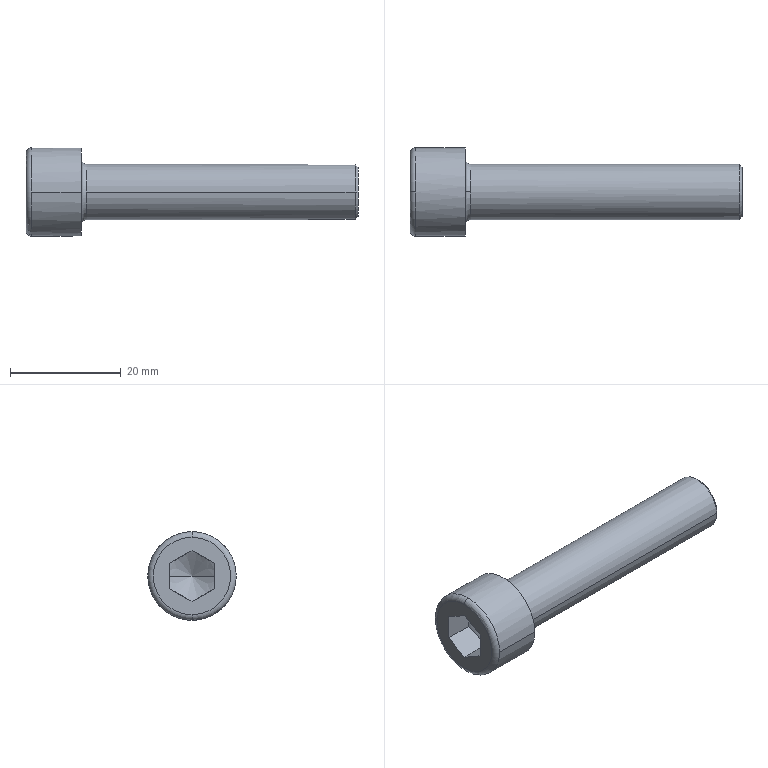Part | NX | features MOVE_FACE 5, BREP 1 | 1 solid | 21 faces | box 60 x 16 x 16 mm | volume 5595 mm3 | plane 9 | cylinder 4 | torus 4 | cone 4 | commonest cylinder face diameters 10 x2 16 x2
STEP:
#1=CARTESIAN_POINT('',(-9.,8.,0.));
#2=VERTEX_POINT('',#1);
#3=CARTESIAN_POINT('',(0.,8.,0.));
#4=VERTEX_POINT('',#3);
#5=CARTESIAN_POINT('',(-4.5,8.,0.));
#6=DIRECTION('',(1.,0.,0.));
#7=VECTOR('',#6,1000.);
#8=LINE('',#5,#7);
#9=EDGE_CURVE('',#2,#4,#8,.T.);
#10=ORIENTED_EDGE('',*,*,#9,.F.);
#11=CARTESIAN_POINT('',(-9.,0.,8.));
#12=VERTEX_POINT('',#11);
#13=CARTESIAN_POINT('',(-9.,0.,0.));
#14=DIRECTION('',(1.,0.,0.));
#15=DIRECTION('',(0.,1.,0.));
#16=AXIS2_PLACEMENT_3D('',#13,#14,#15);
#17=CIRCLE('',#16,8.);
#18=EDGE_CURVE('',#2,#12,#17,.T.);
#19=ORIENTED_EDGE('',*,*,#18,.T.);
#20=CARTESIAN_POINT('',(-9.,-8.,0.));
#21=VERTEX_POINT('',#20);
#22=CARTESIAN_POINT('',(-9.,0.,0.));
#23=DIRECTION('',(1.,0.,0.));
#24=DIRECTION('',(0.,1.,0.));
#25=AXIS2_PLACEMENT_3D('',#22,#23,#24);
#26=CIRCLE('',#25,8.);
#27=EDGE_CURVE('',#12,#21,#26,.T.);
#28=ORIENTED_EDGE('',*,*,#27,.T.);
#29=CARTESIAN_POINT('',(0.,-8.,0.));
#30=VERTEX_POINT('',#29);
#31=CARTESIAN_POINT('',(-4.5,-8.,0.));
#32=DIRECTION('',(-1.,0.,0.));
#33=VECTOR('',#32,1000.);
#34=LINE('',#31,#33);
#35=EDGE_CURVE('',#30,#21,#34,.T.);
#36=ORIENTED_EDGE('',*,*,#35,.F.);
#37=CARTESIAN_POINT('',(0.,0.,0.));
#38=DIRECTION('',(1.,0.,0.));
#39=DIRECTION('',(0.,1.,0.));
#40=AXIS2_PLACEMENT_3D('',#37,#38,#39);
#41=CIRCLE('',#40,8.);
#42=EDGE_CURVE('',#4,#30,#41,.T.);
#43=ORIENTED_EDGE('',*,*,#42,.F.);
#44=EDGE_LOOP('',(#10,#19,#28,#36,#43));
#45=FACE_BOUND('',#44,.T.);
#46=CARTESIAN_POINT('',(-4.5,0.,0.));
#47=DIRECTION('',(1.,0.,0.));
#48=DIRECTION('',(0.,-1.,0.));
#49=AXIS2_PLACEMENT_3D('',#46,#47,#48);
#50=CYLINDRICAL_SURFACE('',#49,8.);
#51=ADVANCED_FACE('',(#45),#50,.T.);
#52=CARTESIAN_POINT('',(-10.,0.,-7.));
#53=VERTEX_POINT('',#52);
#54=CARTESIAN_POINT('',(-9.,0.,-8.));
#55=VERTEX_POINT('',#54);
#56=CARTESIAN_POINT('',(-9.,0.,-7.));
#57=DIRECTION('',(0.,-1.,0.));
#58=DIRECTION('',(0.,0.,-1.));
#59=AXIS2_PLACEMENT_3D('',#56,#57,#58);
#60=CIRCLE('',#59,1.);
#61=EDGE_CURVE('',#53,#55,#60,.T.);
#62=ORIENTED_EDGE('',*,*,#61,.F.);
#63=CARTESIAN_POINT('',(-10.,7.,0.));
#64=VERTEX_POINT('',#63);
#65=CARTESIAN_POINT('',(-10.,0.,0.));
#66=DIRECTION('',(1.,0.,0.));
#67=DIRECTION('',(0.,1.,0.));
#68=AXIS2_PLACEMENT_3D('',#65,#66,#67);
#69=CIRCLE('',#68,7.);
#70=EDGE_CURVE('',#53,#64,#69,.T.);
#71=ORIENTED_EDGE('',*,*,#70,.T.);
#72=CARTESIAN_POINT('',(-10.,0.,7.));
#73=VERTEX_POINT('',#72);
#74=CARTESIAN_POINT('',(-10.,0.,0.));
#75=DIRECTION('',(1.,0.,0.));
#76=DIRECTION('',(0.,1.,0.));
#77=AXIS2_PLACEMENT_3D('',#74,#75,#76);
#78=CIRCLE('',#77,7.);
#79=EDGE_CURVE('',#64,#73,#78,.T.);
#80=ORIENTED_EDGE('',*,*,#79,.T.);
#81=CARTESIAN_POINT('',(-9.,0.,7.));
#82=DIRECTION('',(0.,-1.,0.));
#83=DIRECTION('',(0.,0.,1.));
#84=AXIS2_PLACEMENT_3D('',#81,#82,#83);
#85=CIRCLE('',#84,1.);
#86=EDGE_CURVE('',#12,#73,#85,.T.);
#87=ORIENTED_EDGE('',*,*,#86,.F.);
#88=ORIENTED_EDGE('',*,*,#18,.F.);
#89=CARTESIAN_POINT('',(-9.,0.,0.));
#90=DIRECTION('',(1.,0.,0.));
#91=DIRECTION('',(0.,1.,0.));
#92=AXIS2_PLACEMENT_3D('',#89,#90,#91);
#93=CIRCLE('',#92,8.);
#94=EDGE_CURVE('',#55,#2,#93,.T.);
#95=ORIENTED_EDGE('',*,*,#94,.F.);
#96=EDGE_LOOP('',(#62,#71,#80,#87,#88,#95));
#97=FACE_BOUND('',#96,.T.);
#98=CARTESIAN_POINT('',(-9.,0.,0.));
#99=DIRECTION('',(1.,0.,0.));
#100=DIRECTION('',(0.,0.,1.));
#101=AXIS2_PLACEMENT_3D('',#98,#99,#100);
#102=TOROIDAL_SURFACE('',#101,7.,1.);
#103=ADVANCED_FACE('',(#97),#102,.T.);
#104=CARTESIAN_POINT('',(49.459,5.,0.));
#105=VERTEX_POINT('',#104);
#106=CARTESIAN_POINT('',(50.,4.459,0.));
#107=VERTEX_POINT('',#106);
#108=CARTESIAN_POINT('',(49.729,4.729,0.));
#109=DIRECTION('',(0.7071,-0.7071,0.));
#110=VECTOR('',#109,1000.);
#111=LINE('',#108,#110);
#112=EDGE_CURVE('',#105,#107,#111,.T.);
#113=ORIENTED_EDGE('',*,*,#112,.F.);
#114=CARTESIAN_POINT('',(49.459,-5.,0.));
#115=VERTEX_POINT('',#114);
#116=CARTESIAN_POINT('',(49.459,0.,0.));
#117=DIRECTION('',(1.,0.,0.));
#118=DIRECTION('',(0.,1.,0.));
#119=AXIS2_PLACEMENT_3D('',#116,#117,#118);
#120=CIRCLE('',#119,5.);
#121=EDGE_CURVE('',#105,#115,#120,.T.);
#122=ORIENTED_EDGE('',*,*,#121,.T.);
#123=CARTESIAN_POINT('',(50.,-4.459,0.));
#124=VERTEX_POINT('',#123);
#125=CARTESIAN_POINT('',(49.729,-4.729,0.));
#126=DIRECTION('',(-0.7071,-0.7071,0.));
#127=VECTOR('',#126,1000.);
#128=LINE('',#125,#127);
#129=EDGE_CURVE('',#124,#115,#128,.T.);
#130=ORIENTED_EDGE('',*,*,#129,.F.);
#131=CARTESIAN_POINT('',(50.,0.,0.));
#132=DIRECTION('',(1.,0.,0.));
#133=DIRECTION('',(0.,1.,0.));
#134=AXIS2_PLACEMENT_3D('',#131,#132,#133);
#135=CIRCLE('',#134,4.459);
#136=EDGE_CURVE('',#107,#124,#135,.T.);
#137=ORIENTED_EDGE('',*,*,#136,.F.);
#138=EDGE_LOOP('',(#113,#122,#130,#137));
#139=FACE_BOUND('',#138,.T.);
#140=CARTESIAN_POINT('',(49.729,0.,0.));
#141=DIRECTION('',(-1.,0.,0.));
#142=DIRECTION('',(0.,-1.,0.));
#143=AXIS2_PLACEMENT_3D('',#140,#141,#142);
#144=CONICAL_SURFACE('',#143,4.729,0.7854);
#145=ADVANCED_FACE('',(#139),#144,.T.);
#146=CARTESIAN_POINT('',(1.,5.,0.));
#147=VERTEX_POINT('',#146);
#148=CARTESIAN_POINT('',(8.229,5.,0.));
#149=DIRECTION('',(1.,0.,0.));
#150=VECTOR('',#149,1000.);
#151=LINE('',#148,#150);
#152=EDGE_CURVE('',#147,#105,#151,.T.);
#153=ORIENTED_EDGE('',*,*,#152,.F.);
#154=CARTESIAN_POINT('',(1.,0.,5.));
#155=VERTEX_POINT('',#154);
#156=CARTESIAN_POINT('',(1.,0.,0.));
#157=DIRECTION('',(1.,0.,0.));
#158=DIRECTION('',(0.,1.,0.));
#159=AXIS2_PLACEMENT_3D('',#156,#157,#158);
#160=CIRCLE('',#159,5.);
#161=EDGE_CURVE('',#147,#155,#160,.T.);
#162=ORIENTED_EDGE('',*,*,#161,.T.);
#163=CARTESIAN_POINT('',(1.,-5.,0.));
#164=VERTEX_POINT('',#163);
#165=CARTESIAN_POINT('',(1.,0.,0.));
#166=DIRECTION('',(1.,0.,0.));
#167=DIRECTION('',(0.,1.,0.));
#168=AXIS2_PLACEMENT_3D('',#165,#166,#167);
#169=CIRCLE('',#168,5.);
#170=EDGE_CURVE('',#155,#164,#169,.T.);
#171=ORIENTED_EDGE('',*,*,#170,.T.);
#172=CARTESIAN_POINT('',(8.229,-5.,0.));
#173=DIRECTION('',(-1.,0.,0.));
#174=VECTOR('',#173,1000.);
#175=LINE('',#172,#174);
#176=EDGE_CURVE('',#115,#164,#175,.T.);
#177=ORIENTED_EDGE('',*,*,#176,.F.);
#178=ORIENTED_EDGE('',*,*,#121,.F.);
#179=EDGE_LOOP('',(#153,#162,#171,#177,#178));
#180=FACE_BOUND('',#179,.T.);
#181=CARTESIAN_POINT('',(8.229,0.,0.));
#182=DIRECTION('',(1.,0.,0.));
#183=DIRECTION('',(0.,-1.,0.));
#184=AXIS2_PLACEMENT_3D('',#181,#182,#183);
#185=CYLINDRICAL_SURFACE('',#184,5.);
#186=ADVANCED_FACE('',(#180),#185,.T.);
#187=CARTESIAN_POINT('',(0.,0.,6.));
#188=VERTEX_POINT('',#187);
#189=CARTESIAN_POINT('',(1.,0.,6.));
#190=DIRECTION('',(0.,-1.,0.));
#191=DIRECTION('',(0.,0.,1.));
#192=AXIS2_PLACEMENT_3D('',#189,#190,#191);
#193=CIRCLE('',#192,1.);
#194=EDGE_CURVE('',#188,#155,#193,.T.);
#195=ORIENTED_EDGE('',*,*,#194,.F.);
#196=CARTESIAN_POINT('',(0.,0.,-6.));
#197=VERTEX_POINT('',#196);
#198=CARTESIAN_POINT('',(0.,0.,0.));
#199=DIRECTION('',(1.,0.,0.));
#200=DIRECTION('',(0.,1.,0.));
#201=AXIS2_PLACEMENT_3D('',#198,#199,#200);
#202=CIRCLE('',#201,6.);
#203=EDGE_CURVE('',#188,#197,#202,.T.);
#204=ORIENTED_EDGE('',*,*,#203,.T.);
#205=CARTESIAN_POINT('',(1.,0.,-5.));
#206=VERTEX_POINT('',#205);
#207=CARTESIAN_POINT('',(1.,0.,-6.));
#208=DIRECTION('',(0.,-1.,0.));
#209=DIRECTION('',(0.,0.,-1.));
#210=AXIS2_PLACEMENT_3D('',#207,#208,#209);
#211=CIRCLE('',#210,1.);
#212=EDGE_CURVE('',#206,#197,#211,.T.);
#213=ORIENTED_EDGE('',*,*,#212,.F.);
#214=CARTESIAN_POINT('',(1.,0.,0.));
#215=DIRECTION('',(1.,0.,0.));
#216=DIRECTION('',(0.,1.,0.));
#217=AXIS2_PLACEMENT_3D('',#214,#215,#216);
#218=CIRCLE('',#217,5.);
#219=EDGE_CURVE('',#164,#206,#218,.T.);
#220=ORIENTED_EDGE('',*,*,#219,.F.);
#221=ORIENTED_EDGE('',*,*,#170,.F.);
#222=EDGE_LOOP('',(#195,#204,#213,#220,#221));
#223=FACE_BOUND('',#222,.T.);
#224=CARTESIAN_POINT('',(1.,0.,0.));
#225=DIRECTION('',(1.,0.,0.));
#226=DIRECTION('',(0.,0.,1.));
#227=AXIS2_PLACEMENT_3D('',#224,#225,#226);
#228=TOROIDAL_SURFACE('',#227,6.,1.);
#229=ADVANCED_FACE('',(#223),#228,.F.);
#230=CARTESIAN_POINT('',(-4.644,-4.001,0.));
#231=VERTEX_POINT('',#230);
#232=CARTESIAN_POINT('',(-2.334,0.,0.));
#233=VERTEX_POINT('',#232);
#234=CARTESIAN_POINT('',(-3.667,-2.31,0.));
#235=DIRECTION('',(0.5,0.866,0.));
#236=VECTOR('',#235,1000.);
#237=LINE('',#234,#236);
#238=EDGE_CURVE('',#231,#233,#237,.T.);
#239=ORIENTED_EDGE('',*,*,#238,.T.);
#240=CARTESIAN_POINT('',(-4.644,4.001,0.));
#241=VERTEX_POINT('',#240);
#242=CARTESIAN_POINT('',(-3.667,2.31,0.));
#243=DIRECTION('',(-0.5,0.866,0.));
#244=VECTOR('',#243,1000.);
#245=LINE('',#242,#244);
#246=EDGE_CURVE('',#233,#241,#245,.T.);
#247=ORIENTED_EDGE('',*,*,#246,.T.);
#248=CARTESIAN_POINT('',(-5.001,4.001,-2.31));
#249=VERTEX_POINT('',#248);
#250=CARTESIAN_POINT('',(-5.001,4.001,2.31));
#251=CARTESIAN_POINT('',(-4.334,4.001,0.));
#252=CARTESIAN_POINT('',(-5.001,4.001,-2.31));
#253=(BOUNDED_CURVE()B_SPLINE_CURVE(2,(#250,#251,#252),.UNSPECIFIED.,.F.,.F.)B_SPLINE_CURVE_WITH_KNOTS((3,3),(0.,1.),.PIECEWISE_BEZIER_KNOTS.)CURVE()GEOMETRIC_REPRESENTATION_ITEM()RATIONAL_B_SPLINE_CURVE((1.,1.155,1.))REPRESENTATION_ITEM(''));
#254=EDGE_CURVE('',#241,#249,#253,.T.);
#255=ORIENTED_EDGE('',*,*,#254,.T.);
#256=CARTESIAN_POINT('',(-5.001,0.,-4.62));
#257=VERTEX_POINT('',#256);
#258=CARTESIAN_POINT('',(-5.001,4.001,-2.31));
#259=CARTESIAN_POINT('',(-4.334,2.001,-3.465));
#260=CARTESIAN_POINT('',(-5.001,0.,-4.62));
#261=(BOUNDED_CURVE()B_SPLINE_CURVE(2,(#258,#259,#260),.UNSPECIFIED.,.F.,.F.)B_SPLINE_CURVE_WITH_KNOTS((3,3),(0.,1.),.PIECEWISE_BEZIER_KNOTS.)CURVE()GEOMETRIC_REPRESENTATION_ITEM()RATIONAL_B_SPLINE_CURVE((1.,1.155,1.))REPRESENTATION_ITEM(''));
#262=EDGE_CURVE('',#249,#257,#261,.T.);
#263=ORIENTED_EDGE('',*,*,#262,.T.);
#264=CARTESIAN_POINT('',(-5.001,-4.001,-2.31));
#265=VERTEX_POINT('',#264);
#266=CARTESIAN_POINT('',(-5.001,0.,-4.62));
#267=CARTESIAN_POINT('',(-4.334,-2.001,-3.465));
#268=CARTESIAN_POINT('',(-5.001,-4.001,-2.31));
#269=(BOUNDED_CURVE()B_SPLINE_CURVE(2,(#266,#267,#268),.UNSPECIFIED.,.F.,.F.)B_SPLINE_CURVE_WITH_KNOTS((3,3),(0.,1.),.PIECEWISE_BEZIER_KNOTS.)CURVE()GEOMETRIC_REPRESENTATION_ITEM()RATIONAL_B_SPLINE_CURVE((1.,1.155,1.))REPRESENTATION_ITEM(''));
#270=EDGE_CURVE('',#257,#265,#269,.T.);
#271=ORIENTED_EDGE('',*,*,#270,.T.);
#272=CARTESIAN_POINT('',(-5.001,-4.001,-2.31));
#273=CARTESIAN_POINT('',(-4.334,-4.001,0.));
#274=CARTESIAN_POINT('',(-5.001,-4.001,2.31));
#275=(BOUNDED_CURVE()B_SPLINE_CURVE(2,(#272,#273,#274),.UNSPECIFIED.,.F.,.F.)B_SPLINE_CURVE_WITH_KNOTS((3,3),(0.,1.),.PIECEWISE_BEZIER_KNOTS.)CURVE()GEOMETRIC_REPRESENTATION_ITEM()RATIONAL_B_SPLINE_CURVE((1.,1.155,1.))REPRESENTATION_ITEM(''));
#276=EDGE_CURVE('',#265,#231,#275,.T.);
#277=ORIENTED_EDGE('',*,*,#276,.T.);
#278=EDGE_LOOP('',(#239,#247,#255,#263,#271,#277));
#279=FACE_BOUND('',#278,.T.);
#280=CARTESIAN_POINT('',(-3.667,0.,0.));
#281=DIRECTION('',(-1.,0.,0.));
#282=DIRECTION('',(0.,-1.,0.));
#283=AXIS2_PLACEMENT_3D('',#280,#281,#282);
#284=CONICAL_SURFACE('',#283,2.31,1.047);
#285=ADVANCED_FACE('',(#279),#284,.F.);
#286=CARTESIAN_POINT('',(-10.,-4.001,-2.31));
#287=VERTEX_POINT('',#286);
#288=CARTESIAN_POINT('',(-10.,0.,-4.62));
#289=VERTEX_POINT('',#288);
#290=CARTESIAN_POINT('',(-10.,-0.688,-4.223));
#291=DIRECTION('',(0.,0.866,-0.5));
#292=VECTOR('',#291,1000.);
#293=LINE('',#290,#292);
#294=EDGE_CURVE('',#287,#289,#293,.T.);
#295=ORIENTED_EDGE('',*,*,#294,.F.);
#296=CARTESIAN_POINT('',(-7.501,-4.001,-2.31));
#297=DIRECTION('',(-1.,0.,0.));
#298=VECTOR('',#297,1000.);
#299=LINE('',#296,#298);
#300=EDGE_CURVE('',#265,#287,#299,.T.);
#301=ORIENTED_EDGE('',*,*,#300,.F.);
#302=ORIENTED_EDGE('',*,*,#270,.F.);
#303=CARTESIAN_POINT('',(-7.501,0.,-4.62));
#304=DIRECTION('',(-1.,0.,0.));
#305=VECTOR('',#304,1000.);
#306=LINE('',#303,#305);
#307=EDGE_CURVE('',#257,#289,#306,.T.);
#308=ORIENTED_EDGE('',*,*,#307,.T.);
#309=EDGE_LOOP('',(#295,#301,#302,#308));
#310=FACE_BOUND('',#309,.T.);
#311=CARTESIAN_POINT('',(-10.001,-2.001,-3.465));
#312=DIRECTION('',(0.,-0.5,-0.866));
#313=DIRECTION('',(0.,-0.866,0.5));
#314=AXIS2_PLACEMENT_3D('',#311,#312,#313);
#315=PLANE('',#314);
#316=ADVANCED_FACE('',(#310),#315,.F.);
#317=CARTESIAN_POINT('',(-10.,4.001,-2.31));
#318=VERTEX_POINT('',#317);
#319=CARTESIAN_POINT('',(-10.,3.313,-2.707));
#320=DIRECTION('',(0.,0.866,0.5));
#321=VECTOR('',#320,1000.);
#322=LINE('',#319,#321);
#323=EDGE_CURVE('',#289,#318,#322,.T.);
#324=ORIENTED_EDGE('',*,*,#323,.F.);
#325=ORIENTED_EDGE('',*,*,#307,.F.);
#326=ORIENTED_EDGE('',*,*,#262,.F.);
#327=CARTESIAN_POINT('',(-7.501,4.001,-2.31));
#328=DIRECTION('',(-1.,0.,0.));
#329=VECTOR('',#328,1000.);
#330=LINE('',#327,#329);
#331=EDGE_CURVE('',#249,#318,#330,.T.);
#332=ORIENTED_EDGE('',*,*,#331,.T.);
#333=EDGE_LOOP('',(#324,#325,#326,#332));
#334=FACE_BOUND('',#333,.T.);
#335=CARTESIAN_POINT('',(-10.001,2.001,-3.465));
#336=DIRECTION('',(0.,0.5,-0.866));
#337=DIRECTION('',(0.,-0.866,-0.5));
#338=AXIS2_PLACEMENT_3D('',#335,#336,#337);
#339=PLANE('',#338);
#340=ADVANCED_FACE('',(#334),#339,.F.);
#341=CARTESIAN_POINT('',(-10.,4.001,2.31));
#342=VERTEX_POINT('',#341);
#343=CARTESIAN_POINT('',(-10.,4.001,0.));
#344=DIRECTION('',(0.,0.,1.));
#345=VECTOR('',#344,1000.);
#346=LINE('',#343,#345);
#347=EDGE_CURVE('',#318,#342,#346,.T.);
#348=ORIENTED_EDGE('',*,*,#347,.F.);
#349=ORIENTED_EDGE('',*,*,#331,.F.);
#350=ORIENTED_EDGE('',*,*,#254,.F.);
#351=CARTESIAN_POINT('',(-5.001,4.001,2.31));
#352=VERTEX_POINT('',#351);
#353=CARTESIAN_POINT('',(-5.001,4.001,2.31));
#354=CARTESIAN_POINT('',(-4.334,4.001,0.));
#355=CARTESIAN_POINT('',(-5.001,4.001,-2.31));
#356=(BOUNDED_CURVE()B_SPLINE_CURVE(2,(#353,#354,#355),.UNSPECIFIED.,.F.,.F.)B_SPLINE_CURVE_WITH_KNOTS((3,3),(0.,1.),.PIECEWISE_BEZIER_KNOTS.)CURVE()GEOMETRIC_REPRESENTATION_ITEM()RATIONAL_B_SPLINE_CURVE((1.,1.155,1.))REPRESENTATION_ITEM(''));
#357=EDGE_CURVE('',#352,#241,#356,.T.);
#358=ORIENTED_EDGE('',*,*,#357,.F.);
#359=CARTESIAN_POINT('',(-7.501,4.001,2.31));
#360=DIRECTION('',(-1.,0.,0.));
#361=VECTOR('',#360,1000.);
#362=LINE('',#359,#361);
#363=EDGE_CURVE('',#352,#342,#362,.T.);
#364=ORIENTED_EDGE('',*,*,#363,.T.);
#365=EDGE_LOOP('',(#348,#349,#350,#358,#364));
#366=FACE_BOUND('',#365,.T.);
#367=CARTESIAN_POINT('',(-10.001,4.001,0.));
#368=DIRECTION('',(0.,1.,0.));
#369=DIRECTION('',(0.,0.,-1.));
#370=AXIS2_PLACEMENT_3D('',#367,#368,#369);
#371=PLANE('',#370);
#372=ADVANCED_FACE('',(#366),#371,.F.);
#373=CARTESIAN_POINT('',(-10.,-4.001,2.31));
#374=VERTEX_POINT('',#373);
#375=CARTESIAN_POINT('',(-10.,-4.001,0.));
#376=DIRECTION('',(0.,0.,-1.));
#377=VECTOR('',#376,1000.);
#378=LINE('',#375,#377);
#379=EDGE_CURVE('',#374,#287,#378,.T.);
#380=ORIENTED_EDGE('',*,*,#379,.F.);
#381=CARTESIAN_POINT('',(-5.001,-4.001,2.31));
#382=VERTEX_POINT('',#381);
#383=CARTESIAN_POINT('',(-7.501,-4.001,2.31));
#384=DIRECTION('',(-1.,0.,0.));
#385=VECTOR('',#384,1000.);
#386=LINE('',#383,#385);
#387=EDGE_CURVE('',#382,#374,#386,.T.);
#388=ORIENTED_EDGE('',*,*,#387,.F.);
#389=CARTESIAN_POINT('',(-5.001,-4.001,-2.31));
#390=CARTESIAN_POINT('',(-4.334,-4.001,0.));
#391=CARTESIAN_POINT('',(-5.001,-4.001,2.31));
#392=(BOUNDED_CURVE()B_SPLINE_CURVE(2,(#389,#390,#391),.UNSPECIFIED.,.F.,.F.)B_SPLINE_CURVE_WITH_KNOTS((3,3),(0.,1.),.PIECEWISE_BEZIER_KNOTS.)CURVE()GEOMETRIC_REPRESENTATION_ITEM()RATIONAL_B_SPLINE_CURVE((1.,1.155,1.))REPRESENTATION_ITEM(''));
#393=EDGE_CURVE('',#231,#382,#392,.T.);
#394=ORIENTED_EDGE('',*,*,#393,.F.);
#395=ORIENTED_EDGE('',*,*,#276,.F.);
#396=ORIENTED_EDGE('',*,*,#300,.T.);
#397=EDGE_LOOP('',(#380,#388,#394,#395,#396));
#398=FACE_BOUND('',#397,.T.);
#399=CARTESIAN_POINT('',(-10.001,-4.001,0.));
#400=DIRECTION('',(0.,-1.,0.));
#401=DIRECTION('',(0.,0.,1.));
#402=AXIS2_PLACEMENT_3D('',#399,#400,#401);
#403=PLANE('',#402);
#404=ADVANCED_FACE('',(#398),#403,.F.);
#405=CARTESIAN_POINT('',(-10.,0.,4.62));
#406=VERTEX_POINT('',#405);
#407=CARTESIAN_POINT('',(-10.,3.313,2.707));
#408=DIRECTION('',(0.,-0.866,0.5));
#409=VECTOR('',#408,1000.);
#410=LINE('',#407,#409);
#411=EDGE_CURVE('',#342,#406,#410,.T.);
#412=ORIENTED_EDGE('',*,*,#411,.F.);
#413=ORIENTED_EDGE('',*,*,#363,.F.);
#414=CARTESIAN_POINT('',(-5.001,0.,4.62));
#415=VERTEX_POINT('',#414);
#416=CARTESIAN_POINT('',(-5.001,0.,4.62));
#417=CARTESIAN_POINT('',(-4.334,2.001,3.465));
#418=CARTESIAN_POINT('',(-5.001,4.001,2.31));
#419=(BOUNDED_CURVE()B_SPLINE_CURVE(2,(#416,#417,#418),.UNSPECIFIED.,.F.,.F.)B_SPLINE_CURVE_WITH_KNOTS((3,3),(0.,1.),.PIECEWISE_BEZIER_KNOTS.)CURVE()GEOMETRIC_REPRESENTATION_ITEM()RATIONAL_B_SPLINE_CURVE((1.,1.155,1.))REPRESENTATION_ITEM(''));
#420=EDGE_CURVE('',#415,#352,#419,.T.);
#421=ORIENTED_EDGE('',*,*,#420,.F.);
#422=CARTESIAN_POINT('',(-7.501,0.,4.62));
#423=DIRECTION('',(1.,0.,0.));
#424=VECTOR('',#423,1000.);
#425=LINE('',#422,#424);
#426=EDGE_CURVE('',#406,#415,#425,.T.);
#427=ORIENTED_EDGE('',*,*,#426,.F.);
#428=EDGE_LOOP('',(#412,#413,#421,#427));
#429=FACE_BOUND('',#428,.T.);
#430=CARTESIAN_POINT('',(-10.001,2.001,3.465));
#431=DIRECTION('',(0.,0.5,0.866));
#432=DIRECTION('',(0.,0.866,-0.5));
#433=AXIS2_PLACEMENT_3D('',#430,#431,#432);
#434=PLANE('',#433);
#435=ADVANCED_FACE('',(#429),#434,.F.);
#436=CARTESIAN_POINT('',(-10.,-0.688,4.223));
#437=DIRECTION('',(0.,-0.866,-0.5));
#438=VECTOR('',#437,1000.);
#439=LINE('',#436,#438);
#440=EDGE_CURVE('',#406,#374,#439,.T.);
#441=ORIENTED_EDGE('',*,*,#440,.F.);
#442=ORIENTED_EDGE('',*,*,#426,.T.);
#443=CARTESIAN_POINT('',(-5.001,-4.001,2.31));
#444=CARTESIAN_POINT('',(-4.334,-2.001,3.465));
#445=CARTESIAN_POINT('',(-5.001,0.,4.62));
#446=(BOUNDED_CURVE()B_SPLINE_CURVE(2,(#443,#444,#445),.UNSPECIFIED.,.F.,.F.)B_SPLINE_CURVE_WITH_KNOTS((3,3),(0.,1.),.PIECEWISE_BEZIER_KNOTS.)CURVE()GEOMETRIC_REPRESENTATION_ITEM()RATIONAL_B_SPLINE_CURVE((1.,1.155,1.))REPRESENTATION_ITEM(''));
#447=EDGE_CURVE('',#382,#415,#446,.T.);
#448=ORIENTED_EDGE('',*,*,#447,.F.);
#449=ORIENTED_EDGE('',*,*,#387,.T.);
#450=EDGE_LOOP('',(#441,#442,#448,#449));
#451=FACE_BOUND('',#450,.T.);
#452=CARTESIAN_POINT('',(-10.001,-2.001,3.465));
#453=DIRECTION('',(0.,-0.5,0.866));
#454=DIRECTION('',(0.,0.866,0.5));
#455=AXIS2_PLACEMENT_3D('',#452,#453,#454);
#456=PLANE('',#455);
#457=ADVANCED_FACE('',(#451),#456,.F.);
#458=ORIENTED_EDGE('',*,*,#238,.F.);
#459=ORIENTED_EDGE('',*,*,#393,.T.);
#460=ORIENTED_EDGE('',*,*,#447,.T.);
#461=ORIENTED_EDGE('',*,*,#420,.T.);
#462=ORIENTED_EDGE('',*,*,#357,.T.);
#463=ORIENTED_EDGE('',*,*,#246,.F.);
#464=EDGE_LOOP('',(#458,#459,#460,#461,#462,#463));
#465=FACE_BOUND('',#464,.T.);
#466=CARTESIAN_POINT('',(-3.667,0.,0.));
#467=DIRECTION('',(-1.,0.,0.));
#468=DIRECTION('',(0.,-1.,0.));
#469=AXIS2_PLACEMENT_3D('',#466,#467,#468);
#470=CONICAL_SURFACE('',#469,2.31,1.047);
#471=ADVANCED_FACE('',(#465),#470,.F.);
#472=ORIENTED_EDGE('',*,*,#194,.T.);
#473=ORIENTED_EDGE('',*,*,#161,.F.);
#474=CARTESIAN_POINT('',(1.,0.,0.));
#475=DIRECTION('',(1.,0.,0.));
#476=DIRECTION('',(0.,1.,0.));
#477=AXIS2_PLACEMENT_3D('',#474,#475,#476);
#478=CIRCLE('',#477,5.);
#479=EDGE_CURVE('',#206,#147,#478,.T.);
#480=ORIENTED_EDGE('',*,*,#479,.F.);
#481=ORIENTED_EDGE('',*,*,#212,.T.);
#482=CARTESIAN_POINT('',(0.,6.,0.));
#483=VERTEX_POINT('',#482);
#484=CARTESIAN_POINT('',(0.,0.,0.));
#485=DIRECTION('',(1.,0.,0.));
#486=DIRECTION('',(0.,1.,0.));
#487=AXIS2_PLACEMENT_3D('',#484,#485,#486);
#488=CIRCLE('',#487,6.);
#489=EDGE_CURVE('',#197,#483,#488,.T.);
#490=ORIENTED_EDGE('',*,*,#489,.T.);
#491=CARTESIAN_POINT('',(0.,0.,0.));
#492=DIRECTION('',(1.,0.,0.));
#493=DIRECTION('',(0.,1.,0.));
#494=AXIS2_PLACEMENT_3D('',#491,#492,#493);
#495=CIRCLE('',#494,6.);
#496=EDGE_CURVE('',#483,#188,#495,.T.);
#497=ORIENTED_EDGE('',*,*,#496,.T.);
#498=EDGE_LOOP('',(#472,#473,#480,#481,#490,#497));
#499=FACE_BOUND('',#498,.T.);
#500=CARTESIAN_POINT('',(1.,0.,0.));
#501=DIRECTION('',(1.,0.,0.));
#502=DIRECTION('',(0.,0.,1.));
#503=AXIS2_PLACEMENT_3D('',#500,#501,#502);
#504=TOROIDAL_SURFACE('',#503,6.,1.);
#505=ADVANCED_FACE('',(#499),#504,.F.);
#506=ORIENTED_EDGE('',*,*,#152,.T.);
#507=CARTESIAN_POINT('',(49.459,0.,0.));
#508=DIRECTION('',(1.,0.,0.));
#509=DIRECTION('',(0.,1.,0.));
#510=AXIS2_PLACEMENT_3D('',#507,#508,#509);
#511=CIRCLE('',#510,5.);
#512=EDGE_CURVE('',#115,#105,#511,.T.);
#513=ORIENTED_EDGE('',*,*,#512,.F.);
#514=ORIENTED_EDGE('',*,*,#176,.T.);
#515=ORIENTED_EDGE('',*,*,#219,.T.);
#516=ORIENTED_EDGE('',*,*,#479,.T.);
#517=EDGE_LOOP('',(#506,#513,#514,#515,#516));
#518=FACE_BOUND('',#517,.T.);
#519=CARTESIAN_POINT('',(8.229,0.,0.));
#520=DIRECTION('',(1.,0.,0.));
#521=DIRECTION('',(0.,-1.,0.));
#522=AXIS2_PLACEMENT_3D('',#519,#520,#521);
#523=CYLINDRICAL_SURFACE('',#522,5.);
#524=ADVANCED_FACE('',(#518),#523,.T.);
#525=ORIENTED_EDGE('',*,*,#112,.T.);
#526=CARTESIAN_POINT('',(50.,0.,0.));
#527=DIRECTION('',(1.,0.,0.));
#528=DIRECTION('',(0.,1.,0.));
#529=AXIS2_PLACEMENT_3D('',#526,#527,#528);
#530=CIRCLE('',#529,4.459);
#531=EDGE_CURVE('',#124,#107,#530,.T.);
#532=ORIENTED_EDGE('',*,*,#531,.F.);
#533=ORIENTED_EDGE('',*,*,#129,.T.);
#534=ORIENTED_EDGE('',*,*,#512,.T.);
#535=EDGE_LOOP('',(#525,#532,#533,#534));
#536=FACE_BOUND('',#535,.T.);
#537=CARTESIAN_POINT('',(49.729,0.,0.));
#538=DIRECTION('',(-1.,0.,0.));
#539=DIRECTION('',(0.,-1.,0.));
#540=AXIS2_PLACEMENT_3D('',#537,#538,#539);
#541=CONICAL_SURFACE('',#540,4.729,0.7854);
#542=ADVANCED_FACE('',(#536),#541,.T.);
#543=ORIENTED_EDGE('',*,*,#136,.T.);
#544=ORIENTED_EDGE('',*,*,#531,.T.);
#545=EDGE_LOOP('',(#543,#544));
#546=FACE_BOUND('',#545,.T.);
#547=CARTESIAN_POINT('',(50.,2.229,0.));
#548=DIRECTION('',(1.,0.,0.));
#549=DIRECTION('',(0.,-1.,0.));
#550=AXIS2_PLACEMENT_3D('',#547,#548,#549);
#551=PLANE('',#550);
#552=ADVANCED_FACE('',(#546),#551,.T.);
#553=ORIENTED_EDGE('',*,*,#411,.T.);
#554=ORIENTED_EDGE('',*,*,#440,.T.);
#555=ORIENTED_EDGE('',*,*,#379,.T.);
#556=ORIENTED_EDGE('',*,*,#294,.T.);
#557=ORIENTED_EDGE('',*,*,#323,.T.);
#558=ORIENTED_EDGE('',*,*,#347,.T.);
#559=EDGE_LOOP('',(#553,#554,#555,#556,#557,#558));
#560=FACE_BOUND('',#559,.T.);
#561=ORIENTED_EDGE('',*,*,#79,.F.);
#562=ORIENTED_EDGE('',*,*,#70,.F.);
#563=CARTESIAN_POINT('',(-10.,0.,0.));
#564=DIRECTION('',(1.,0.,0.));
#565=DIRECTION('',(0.,1.,0.));
#566=AXIS2_PLACEMENT_3D('',#563,#564,#565);
#567=CIRCLE('',#566,7.);
#568=EDGE_CURVE('',#73,#53,#567,.T.);
#569=ORIENTED_EDGE('',*,*,#568,.F.);
#570=EDGE_LOOP('',(#561,#562,#569));
#571=FACE_BOUND('',#570,.T.);
#572=CARTESIAN_POINT('',(-10.,3.5,0.));
#573=DIRECTION('',(-1.,0.,0.));
#574=DIRECTION('',(0.,1.,0.));
#575=AXIS2_PLACEMENT_3D('',#572,#573,#574);
#576=PLANE('',#575);
#577=ADVANCED_FACE('',(#560,#571),#576,.T.);
#578=ORIENTED_EDGE('',*,*,#61,.T.);
#579=CARTESIAN_POINT('',(-9.,0.,0.));
#580=DIRECTION('',(1.,0.,0.));
#581=DIRECTION('',(0.,1.,0.));
#582=AXIS2_PLACEMENT_3D('',#579,#580,#581);
#583=CIRCLE('',#582,8.);
#584=EDGE_CURVE('',#21,#55,#583,.T.);
#585=ORIENTED_EDGE('',*,*,#584,.F.);
#586=ORIENTED_EDGE('',*,*,#27,.F.);
#587=ORIENTED_EDGE('',*,*,#86,.T.);
#588=ORIENTED_EDGE('',*,*,#568,.T.);
#589=EDGE_LOOP('',(#578,#585,#586,#587,#588));
#590=FACE_BOUND('',#589,.T.);
#591=CARTESIAN_POINT('',(-9.,0.,0.));
#592=DIRECTION('',(1.,0.,0.));
#593=DIRECTION('',(0.,0.,1.));
#594=AXIS2_PLACEMENT_3D('',#591,#592,#593);
#595=TOROIDAL_SURFACE('',#594,7.,1.);
#596=ADVANCED_FACE('',(#590),#595,.T.);
#597=ORIENTED_EDGE('',*,*,#9,.T.);
#598=CARTESIAN_POINT('',(0.,0.,0.));
#599=DIRECTION('',(1.,0.,0.));
#600=DIRECTION('',(0.,1.,0.));
#601=AXIS2_PLACEMENT_3D('',#598,#599,#600);
#602=CIRCLE('',#601,8.);
#603=EDGE_CURVE('',#30,#4,#602,.T.);
#604=ORIENTED_EDGE('',*,*,#603,.F.);
#605=ORIENTED_EDGE('',*,*,#35,.T.);
#606=ORIENTED_EDGE('',*,*,#584,.T.);
#607=ORIENTED_EDGE('',*,*,#94,.T.);
#608=EDGE_LOOP('',(#597,#604,#605,#606,#607));
#609=FACE_BOUND('',#608,.T.);
#610=CARTESIAN_POINT('',(-4.5,0.,0.));
#611=DIRECTION('',(1.,0.,0.));
#612=DIRECTION('',(0.,-1.,0.));
#613=AXIS2_PLACEMENT_3D('',#610,#611,#612);
#614=CYLINDRICAL_SURFACE('',#613,8.);
#615=ADVANCED_FACE('',(#609),#614,.T.);
#616=ORIENTED_EDGE('',*,*,#496,.F.);
#617=ORIENTED_EDGE('',*,*,#489,.F.);
#618=ORIENTED_EDGE('',*,*,#203,.F.);
#619=EDGE_LOOP('',(#616,#617,#618));
#620=FACE_BOUND('',#619,.T.);
#621=ORIENTED_EDGE('',*,*,#42,.T.);
#622=ORIENTED_EDGE('',*,*,#603,.T.);
#623=EDGE_LOOP('',(#621,#622));
#624=FACE_BOUND('',#623,.T.);
#625=CARTESIAN_POINT('',(0.,7.,0.));
#626=DIRECTION('',(1.,0.,0.));
#627=DIRECTION('',(0.,-1.,0.));
#628=AXIS2_PLACEMENT_3D('',#625,#626,#627);
#629=PLANE('',#628);
#630=ADVANCED_FACE('',(#620,#624),#629,.T.);
#631=CLOSED_SHELL('',(#51,#103,#145,#186,#229,#285,#316,#340,#372,#404,#435,#457,#471,#505,#524,#542,#552,#577,#596,#615,#630));
#632=MANIFOLD_SOLID_BREP('',#631);
#633=(LENGTH_UNIT()NAMED_UNIT(*)SI_UNIT(.MILLI.,.METRE.));
#634=UNCERTAINTY_MEASURE_WITH_UNIT(LENGTH_MEASURE(0.00001),#633,'','');
#635=(NAMED_UNIT(*)PLANE_ANGLE_UNIT()SI_UNIT($,.RADIAN.));
#636=(NAMED_UNIT(*)SI_UNIT($,.STERADIAN.)SOLID_ANGLE_UNIT());
#637=(GEOMETRIC_REPRESENTATION_CONTEXT(3)GLOBAL_UNCERTAINTY_ASSIGNED_CONTEXT((#634))GLOBAL_UNIT_ASSIGNED_CONTEXT((#633,#635,#636))REPRESENTATION_CONTEXT('',''));
#638=ADVANCED_BREP_SHAPE_REPRESENTATION('',(#632),#637);